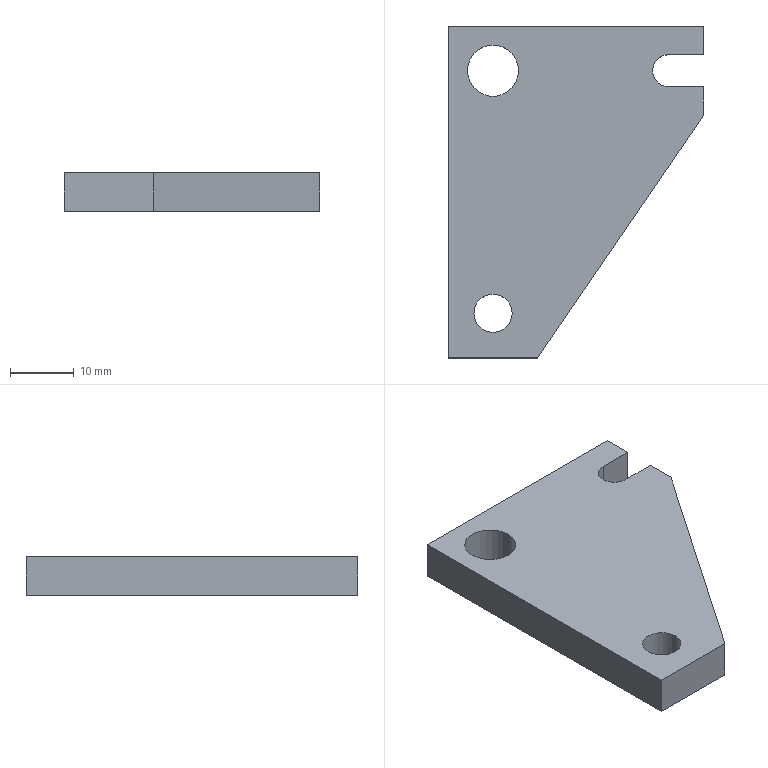Part | STEP file | BU-C03a | 1 solid | 16 faces | box 40 x 52 x 6 mm | volume 8821 mm3 | plane 10 | cylinder 6 | commonest cylinder face diameters 5 x2 6 x2 8 x2
STEP:
#1=CARTESIAN_POINT('',(0.,0.,0.));
#2=DIRECTION('',(0.,0.,1.));
#3=DIRECTION('',(1.,0.,0.));
#4=AXIS2_PLACEMENT_3D('',#1,#2,#3);
#5=CARTESIAN_POINT('',(3.,45.,6.));
#6=VERTEX_POINT('',#5);
#7=CARTESIAN_POINT('',(3.,45.,0.));
#8=VERTEX_POINT('',#7);
#9=CARTESIAN_POINT('',(3.,45.,6.));
#10=DIRECTION('',(0.,0.,-1.));
#11=VECTOR('',#10,1.);
#12=LINE('',#9,#11);
#13=CARTESIAN_POINT('',(7.,45.,6.));
#14=DIRECTION('',(0.,0.,-1.));
#15=DIRECTION('',(-1.,0.,0.));
#16=AXIS2_PLACEMENT_3D('',#13,#14,#15);
#17=CYLINDRICAL_SURFACE('',#16,4.);
#18=CARTESIAN_POINT('',(6.283,0.));
#19=DIRECTION('',(0.,1.));
#20=VECTOR('',#19,1.);
#21=LINE('',#18,#20);
#22=(GEOMETRIC_REPRESENTATION_CONTEXT(2)PARAMETRIC_REPRESENTATION_CONTEXT()REPRESENTATION_CONTEXT('',''));
#23=DEFINITIONAL_REPRESENTATION('',(#21),#22);
#24=PCURVE('',#17,#23);
#25=CARTESIAN_POINT('',(7.,45.,6.));
#26=DIRECTION('',(0.,0.,-1.));
#27=DIRECTION('',(-1.,0.,0.));
#28=AXIS2_PLACEMENT_3D('',#25,#26,#27);
#29=CYLINDRICAL_SURFACE('',#28,4.);
#30=CARTESIAN_POINT('',(0.,0.));
#31=DIRECTION('',(0.,1.));
#32=VECTOR('',#31,1.);
#33=LINE('',#30,#32);
#34=(GEOMETRIC_REPRESENTATION_CONTEXT(2)PARAMETRIC_REPRESENTATION_CONTEXT()REPRESENTATION_CONTEXT('',''));
#35=DEFINITIONAL_REPRESENTATION('',(#33),#34);
#36=PCURVE('',#29,#35);
#37=SURFACE_CURVE('',#12,(#24,#36),.PCURVE_S1.);
#38=EDGE_CURVE('',#6,#8,#37,.T.);
#39=ORIENTED_EDGE('',*,*,#38,.T.);
#40=CARTESIAN_POINT('',(11.,45.,0.));
#41=VERTEX_POINT('',#40);
#42=CARTESIAN_POINT('',(7.,45.,0.));
#43=DIRECTION('',(0.,0.,1.));
#44=DIRECTION('',(1.,0.,0.));
#45=AXIS2_PLACEMENT_3D('',#42,#43,#44);
#46=CIRCLE('',#45,4.);
#47=CARTESIAN_POINT('',(9.425,6.));
#48=DIRECTION('',(-1.,0.));
#49=VECTOR('',#48,1.);
#50=LINE('',#47,#49);
#51=(GEOMETRIC_REPRESENTATION_CONTEXT(2)PARAMETRIC_REPRESENTATION_CONTEXT()REPRESENTATION_CONTEXT('',''));
#52=DEFINITIONAL_REPRESENTATION('',(#50),#51);
#53=PCURVE('',#17,#52);
#54=CARTESIAN_POINT('',(34.5,45.,0.));
#55=DIRECTION('',(0.,0.,1.));
#56=DIRECTION('',(1.,0.,0.));
#57=AXIS2_PLACEMENT_3D('',#54,#55,#56);
#58=PLANE('',#57);
#59=CARTESIAN_POINT('',(-27.5,0.));
#60=DIRECTION('',(1.,0.));
#61=AXIS2_PLACEMENT_2D('',#59,#60);
#62=CIRCLE('',#61,4.);
#63=(GEOMETRIC_REPRESENTATION_CONTEXT(2)PARAMETRIC_REPRESENTATION_CONTEXT()REPRESENTATION_CONTEXT('',''));
#64=DEFINITIONAL_REPRESENTATION('',(#62),#63);
#65=PCURVE('',#58,#64);
#66=SURFACE_CURVE('',#46,(#53,#65),.PCURVE_S1.);
#67=EDGE_CURVE('',#8,#41,#66,.T.);
#68=ORIENTED_EDGE('',*,*,#67,.T.);
#69=CARTESIAN_POINT('',(11.,45.,6.));
#70=VERTEX_POINT('',#69);
#71=CARTESIAN_POINT('',(11.,45.,6.));
#72=DIRECTION('',(0.,0.,-1.));
#73=VECTOR('',#72,1.);
#74=LINE('',#71,#73);
#75=CARTESIAN_POINT('',(3.142,0.));
#76=DIRECTION('',(0.,1.));
#77=VECTOR('',#76,1.);
#78=LINE('',#75,#77);
#79=(GEOMETRIC_REPRESENTATION_CONTEXT(2)PARAMETRIC_REPRESENTATION_CONTEXT()REPRESENTATION_CONTEXT('',''));
#80=DEFINITIONAL_REPRESENTATION('',(#78),#79);
#81=PCURVE('',#17,#80);
#82=CARTESIAN_POINT('',(3.142,0.));
#83=DIRECTION('',(0.,1.));
#84=VECTOR('',#83,1.);
#85=LINE('',#82,#84);
#86=(GEOMETRIC_REPRESENTATION_CONTEXT(2)PARAMETRIC_REPRESENTATION_CONTEXT()REPRESENTATION_CONTEXT('',''));
#87=DEFINITIONAL_REPRESENTATION('',(#85),#86);
#88=PCURVE('',#29,#87);
#89=SURFACE_CURVE('',#74,(#81,#88),.PCURVE_S1.);
#90=EDGE_CURVE('',#70,#41,#89,.T.);
#91=ORIENTED_EDGE('',*,*,#90,.F.);
#92=CARTESIAN_POINT('',(7.,45.,6.));
#93=DIRECTION('',(0.,0.,1.));
#94=DIRECTION('',(1.,0.,0.));
#95=AXIS2_PLACEMENT_3D('',#92,#93,#94);
#96=CIRCLE('',#95,4.);
#97=CARTESIAN_POINT('',(9.425,0.));
#98=DIRECTION('',(-1.,0.));
#99=VECTOR('',#98,1.);
#100=LINE('',#97,#99);
#101=(GEOMETRIC_REPRESENTATION_CONTEXT(2)PARAMETRIC_REPRESENTATION_CONTEXT()REPRESENTATION_CONTEXT('',''));
#102=DEFINITIONAL_REPRESENTATION('',(#100),#101);
#103=PCURVE('',#17,#102);
#104=CARTESIAN_POINT('',(34.5,45.,6.));
#105=DIRECTION('',(0.,0.,1.));
#106=DIRECTION('',(1.,0.,0.));
#107=AXIS2_PLACEMENT_3D('',#104,#105,#106);
#108=PLANE('',#107);
#109=CARTESIAN_POINT('',(-27.5,0.));
#110=DIRECTION('',(1.,0.));
#111=AXIS2_PLACEMENT_2D('',#109,#110);
#112=CIRCLE('',#111,4.);
#113=(GEOMETRIC_REPRESENTATION_CONTEXT(2)PARAMETRIC_REPRESENTATION_CONTEXT()REPRESENTATION_CONTEXT('',''));
#114=DEFINITIONAL_REPRESENTATION('',(#112),#113);
#115=PCURVE('',#108,#114);
#116=SURFACE_CURVE('',#96,(#103,#115),.PCURVE_S1.);
#117=EDGE_CURVE('',#6,#70,#116,.T.);
#118=ORIENTED_EDGE('',*,*,#117,.F.);
#119=EDGE_LOOP('',(#39,#68,#91,#118));
#120=FACE_BOUND('',#119,.F.);
#121=ADVANCED_FACE('',(#120),#17,.F.);
#122=CARTESIAN_POINT('',(4.,7.,6.));
#123=VERTEX_POINT('',#122);
#124=CARTESIAN_POINT('',(4.,7.,0.));
#125=VERTEX_POINT('',#124);
#126=CARTESIAN_POINT('',(4.,7.,6.));
#127=DIRECTION('',(0.,0.,-1.));
#128=VECTOR('',#127,1.);
#129=LINE('',#126,#128);
#130=CARTESIAN_POINT('',(7.,7.,6.));
#131=DIRECTION('',(0.,0.,-1.));
#132=DIRECTION('',(-1.,0.,0.));
#133=AXIS2_PLACEMENT_3D('',#130,#131,#132);
#134=CYLINDRICAL_SURFACE('',#133,3.);
#135=CARTESIAN_POINT('',(6.283,0.));
#136=DIRECTION('',(0.,1.));
#137=VECTOR('',#136,1.);
#138=LINE('',#135,#137);
#139=(GEOMETRIC_REPRESENTATION_CONTEXT(2)PARAMETRIC_REPRESENTATION_CONTEXT()REPRESENTATION_CONTEXT('',''));
#140=DEFINITIONAL_REPRESENTATION('',(#138),#139);
#141=PCURVE('',#134,#140);
#142=CARTESIAN_POINT('',(7.,7.,6.));
#143=DIRECTION('',(0.,0.,-1.));
#144=DIRECTION('',(-1.,0.,0.));
#145=AXIS2_PLACEMENT_3D('',#142,#143,#144);
#146=CYLINDRICAL_SURFACE('',#145,3.);
#147=CARTESIAN_POINT('',(0.,0.));
#148=DIRECTION('',(0.,1.));
#149=VECTOR('',#148,1.);
#150=LINE('',#147,#149);
#151=(GEOMETRIC_REPRESENTATION_CONTEXT(2)PARAMETRIC_REPRESENTATION_CONTEXT()REPRESENTATION_CONTEXT('',''));
#152=DEFINITIONAL_REPRESENTATION('',(#150),#151);
#153=PCURVE('',#146,#152);
#154=SURFACE_CURVE('',#129,(#141,#153),.PCURVE_S1.);
#155=EDGE_CURVE('',#123,#125,#154,.T.);
#156=ORIENTED_EDGE('',*,*,#155,.T.);
#157=CARTESIAN_POINT('',(10.,7.,0.));
#158=VERTEX_POINT('',#157);
#159=CARTESIAN_POINT('',(7.,7.,0.));
#160=DIRECTION('',(0.,0.,1.));
#161=DIRECTION('',(1.,0.,0.));
#162=AXIS2_PLACEMENT_3D('',#159,#160,#161);
#163=CIRCLE('',#162,3.);
#164=CARTESIAN_POINT('',(9.425,6.));
#165=DIRECTION('',(-1.,0.));
#166=VECTOR('',#165,1.);
#167=LINE('',#164,#166);
#168=(GEOMETRIC_REPRESENTATION_CONTEXT(2)PARAMETRIC_REPRESENTATION_CONTEXT()REPRESENTATION_CONTEXT('',''));
#169=DEFINITIONAL_REPRESENTATION('',(#167),#168);
#170=PCURVE('',#134,#169);
#171=CARTESIAN_POINT('',(-27.5,-38.));
#172=DIRECTION('',(1.,0.));
#173=AXIS2_PLACEMENT_2D('',#171,#172);
#174=CIRCLE('',#173,3.);
#175=(GEOMETRIC_REPRESENTATION_CONTEXT(2)PARAMETRIC_REPRESENTATION_CONTEXT()REPRESENTATION_CONTEXT('',''));
#176=DEFINITIONAL_REPRESENTATION('',(#174),#175);
#177=PCURVE('',#58,#176);
#178=SURFACE_CURVE('',#163,(#170,#177),.PCURVE_S1.);
#179=EDGE_CURVE('',#125,#158,#178,.T.);
#180=ORIENTED_EDGE('',*,*,#179,.T.);
#181=CARTESIAN_POINT('',(10.,7.,6.));
#182=VERTEX_POINT('',#181);
#183=CARTESIAN_POINT('',(10.,7.,6.));
#184=DIRECTION('',(0.,0.,-1.));
#185=VECTOR('',#184,1.);
#186=LINE('',#183,#185);
#187=CARTESIAN_POINT('',(3.142,0.));
#188=DIRECTION('',(0.,1.));
#189=VECTOR('',#188,1.);
#190=LINE('',#187,#189);
#191=(GEOMETRIC_REPRESENTATION_CONTEXT(2)PARAMETRIC_REPRESENTATION_CONTEXT()REPRESENTATION_CONTEXT('',''));
#192=DEFINITIONAL_REPRESENTATION('',(#190),#191);
#193=PCURVE('',#134,#192);
#194=CARTESIAN_POINT('',(3.142,0.));
#195=DIRECTION('',(0.,1.));
#196=VECTOR('',#195,1.);
#197=LINE('',#194,#196);
#198=(GEOMETRIC_REPRESENTATION_CONTEXT(2)PARAMETRIC_REPRESENTATION_CONTEXT()REPRESENTATION_CONTEXT('',''));
#199=DEFINITIONAL_REPRESENTATION('',(#197),#198);
#200=PCURVE('',#146,#199);
#201=SURFACE_CURVE('',#186,(#193,#200),.PCURVE_S1.);
#202=EDGE_CURVE('',#182,#158,#201,.T.);
#203=ORIENTED_EDGE('',*,*,#202,.F.);
#204=CARTESIAN_POINT('',(7.,7.,6.));
#205=DIRECTION('',(0.,0.,1.));
#206=DIRECTION('',(1.,0.,0.));
#207=AXIS2_PLACEMENT_3D('',#204,#205,#206);
#208=CIRCLE('',#207,3.);
#209=CARTESIAN_POINT('',(9.425,0.));
#210=DIRECTION('',(-1.,0.));
#211=VECTOR('',#210,1.);
#212=LINE('',#209,#211);
#213=(GEOMETRIC_REPRESENTATION_CONTEXT(2)PARAMETRIC_REPRESENTATION_CONTEXT()REPRESENTATION_CONTEXT('',''));
#214=DEFINITIONAL_REPRESENTATION('',(#212),#213);
#215=PCURVE('',#134,#214);
#216=CARTESIAN_POINT('',(-27.5,-38.));
#217=DIRECTION('',(1.,0.));
#218=AXIS2_PLACEMENT_2D('',#216,#217);
#219=CIRCLE('',#218,3.);
#220=(GEOMETRIC_REPRESENTATION_CONTEXT(2)PARAMETRIC_REPRESENTATION_CONTEXT()REPRESENTATION_CONTEXT('',''));
#221=DEFINITIONAL_REPRESENTATION('',(#219),#220);
#222=PCURVE('',#108,#221);
#223=SURFACE_CURVE('',#208,(#215,#222),.PCURVE_S1.);
#224=EDGE_CURVE('',#123,#182,#223,.T.);
#225=ORIENTED_EDGE('',*,*,#224,.F.);
#226=EDGE_LOOP('',(#156,#180,#203,#225));
#227=FACE_BOUND('',#226,.F.);
#228=ADVANCED_FACE('',(#227),#134,.F.);
#229=CARTESIAN_POINT('',(34.5,47.5,6.));
#230=VERTEX_POINT('',#229);
#231=CARTESIAN_POINT('',(34.5,47.5,0.));
#232=VERTEX_POINT('',#231);
#233=CARTESIAN_POINT('',(34.5,47.5,6.));
#234=DIRECTION('',(0.,0.,-1.));
#235=VECTOR('',#234,1.);
#236=LINE('',#233,#235);
#237=CARTESIAN_POINT('',(34.5,45.,6.));
#238=DIRECTION('',(0.,0.,-1.));
#239=DIRECTION('',(-1.,0.,0.));
#240=AXIS2_PLACEMENT_3D('',#237,#238,#239);
#241=CYLINDRICAL_SURFACE('',#240,2.5);
#242=CARTESIAN_POINT('',(1.571,0.));
#243=DIRECTION('',(0.,1.));
#244=VECTOR('',#243,1.);
#245=LINE('',#242,#244);
#246=(GEOMETRIC_REPRESENTATION_CONTEXT(2)PARAMETRIC_REPRESENTATION_CONTEXT()REPRESENTATION_CONTEXT('',''));
#247=DEFINITIONAL_REPRESENTATION('',(#245),#246);
#248=PCURVE('',#241,#247);
#249=CARTESIAN_POINT('',(40.,47.5,6.));
#250=DIRECTION('',(0.,1.,0.));
#251=DIRECTION('',(0.,0.,1.));
#252=AXIS2_PLACEMENT_3D('',#249,#250,#251);
#253=PLANE('',#252);
#254=CARTESIAN_POINT('',(0.,-5.5));
#255=DIRECTION('',(-1.,0.));
#256=VECTOR('',#255,1.);
#257=LINE('',#254,#256);
#258=(GEOMETRIC_REPRESENTATION_CONTEXT(2)PARAMETRIC_REPRESENTATION_CONTEXT()REPRESENTATION_CONTEXT('',''));
#259=DEFINITIONAL_REPRESENTATION('',(#257),#258);
#260=PCURVE('',#253,#259);
#261=SURFACE_CURVE('',#236,(#248,#260),.PCURVE_S1.);
#262=EDGE_CURVE('',#230,#232,#261,.T.);
#263=ORIENTED_EDGE('',*,*,#262,.T.);
#264=CARTESIAN_POINT('',(32.,45.,0.));
#265=VERTEX_POINT('',#264);
#266=CARTESIAN_POINT('',(34.5,45.,0.));
#267=DIRECTION('',(0.,0.,-1.));
#268=DIRECTION('',(1.,0.,0.));
#269=AXIS2_PLACEMENT_3D('',#266,#267,#268);
#270=CIRCLE('',#269,2.5);
#271=CARTESIAN_POINT('',(-3.142,6.));
#272=DIRECTION('',(1.,0.));
#273=VECTOR('',#272,1.);
#274=LINE('',#271,#273);
#275=(GEOMETRIC_REPRESENTATION_CONTEXT(2)PARAMETRIC_REPRESENTATION_CONTEXT()REPRESENTATION_CONTEXT('',''));
#276=DEFINITIONAL_REPRESENTATION('',(#274),#275);
#277=PCURVE('',#241,#276);
#278=CARTESIAN_POINT('',(2.5,0.));
#279=CARTESIAN_POINT('',(2.5,-4.33));
#280=CARTESIAN_POINT('',(-1.25,-2.165));
#281=CARTESIAN_POINT('',(-5.,0.));
#282=CARTESIAN_POINT('',(-1.25,2.165));
#283=CARTESIAN_POINT('',(2.5,4.33));
#284=CARTESIAN_POINT('',(2.5,0.));
#285=(BOUNDED_CURVE()B_SPLINE_CURVE(2,(#278,#279,#280,#281,#282,#283,#284),.UNSPECIFIED.,.T.,.F.)B_SPLINE_CURVE_WITH_KNOTS((1,2,2,2,2,1),(-2.094,0.,2.094,4.189,6.283,8.378),.UNSPECIFIED.)CURVE()GEOMETRIC_REPRESENTATION_ITEM()RATIONAL_B_SPLINE_CURVE((1.,0.5,1.,0.5,1.,0.5,1.))REPRESENTATION_ITEM(''));
#286=(GEOMETRIC_REPRESENTATION_CONTEXT(2)PARAMETRIC_REPRESENTATION_CONTEXT()REPRESENTATION_CONTEXT('',''));
#287=DEFINITIONAL_REPRESENTATION('',(#285),#286);
#288=PCURVE('',#58,#287);
#289=SURFACE_CURVE('',#270,(#277,#288),.PCURVE_S1.);
#290=EDGE_CURVE('',#265,#232,#289,.T.);
#291=ORIENTED_EDGE('',*,*,#290,.F.);
#292=CARTESIAN_POINT('',(32.,45.,6.));
#293=VERTEX_POINT('',#292);
#294=CARTESIAN_POINT('',(32.,45.,6.));
#295=DIRECTION('',(0.,0.,-1.));
#296=VECTOR('',#295,1.);
#297=LINE('',#294,#296);
#298=CARTESIAN_POINT('',(0.,0.));
#299=DIRECTION('',(0.,1.));
#300=VECTOR('',#299,1.);
#301=LINE('',#298,#300);
#302=(GEOMETRIC_REPRESENTATION_CONTEXT(2)PARAMETRIC_REPRESENTATION_CONTEXT()REPRESENTATION_CONTEXT('',''));
#303=DEFINITIONAL_REPRESENTATION('',(#301),#302);
#304=PCURVE('',#241,#303);
#305=CARTESIAN_POINT('',(34.5,45.,6.));
#306=DIRECTION('',(0.,0.,-1.));
#307=DIRECTION('',(-1.,0.,0.));
#308=AXIS2_PLACEMENT_3D('',#305,#306,#307);
#309=CYLINDRICAL_SURFACE('',#308,2.5);
#310=CARTESIAN_POINT('',(6.283,0.));
#311=DIRECTION('',(0.,1.));
#312=VECTOR('',#311,1.);
#313=LINE('',#310,#312);
#314=(GEOMETRIC_REPRESENTATION_CONTEXT(2)PARAMETRIC_REPRESENTATION_CONTEXT()REPRESENTATION_CONTEXT('',''));
#315=DEFINITIONAL_REPRESENTATION('',(#313),#314);
#316=PCURVE('',#309,#315);
#317=SURFACE_CURVE('',#297,(#304,#316),.PCURVE_S1.);
#318=EDGE_CURVE('',#293,#265,#317,.T.);
#319=ORIENTED_EDGE('',*,*,#318,.F.);
#320=CARTESIAN_POINT('',(34.5,45.,6.));
#321=DIRECTION('',(0.,0.,-1.));
#322=DIRECTION('',(1.,0.,0.));
#323=AXIS2_PLACEMENT_3D('',#320,#321,#322);
#324=CIRCLE('',#323,2.5);
#325=CARTESIAN_POINT('',(-3.142,0.));
#326=DIRECTION('',(1.,0.));
#327=VECTOR('',#326,1.);
#328=LINE('',#325,#327);
#329=(GEOMETRIC_REPRESENTATION_CONTEXT(2)PARAMETRIC_REPRESENTATION_CONTEXT()REPRESENTATION_CONTEXT('',''));
#330=DEFINITIONAL_REPRESENTATION('',(#328),#329);
#331=PCURVE('',#241,#330);
#332=CARTESIAN_POINT('',(2.5,0.));
#333=CARTESIAN_POINT('',(2.5,-4.33));
#334=CARTESIAN_POINT('',(-1.25,-2.165));
#335=CARTESIAN_POINT('',(-5.,0.));
#336=CARTESIAN_POINT('',(-1.25,2.165));
#337=CARTESIAN_POINT('',(2.5,4.33));
#338=CARTESIAN_POINT('',(2.5,0.));
#339=(BOUNDED_CURVE()B_SPLINE_CURVE(2,(#332,#333,#334,#335,#336,#337,#338),.UNSPECIFIED.,.T.,.F.)B_SPLINE_CURVE_WITH_KNOTS((1,2,2,2,2,1),(-2.094,0.,2.094,4.189,6.283,8.378),.UNSPECIFIED.)CURVE()GEOMETRIC_REPRESENTATION_ITEM()RATIONAL_B_SPLINE_CURVE((1.,0.5,1.,0.5,1.,0.5,1.))REPRESENTATION_ITEM(''));
#340=(GEOMETRIC_REPRESENTATION_CONTEXT(2)PARAMETRIC_REPRESENTATION_CONTEXT()REPRESENTATION_CONTEXT('',''));
#341=DEFINITIONAL_REPRESENTATION('',(#339),#340);
#342=PCURVE('',#108,#341);
#343=SURFACE_CURVE('',#324,(#331,#342),.PCURVE_S1.);
#344=EDGE_CURVE('',#293,#230,#343,.T.);
#345=ORIENTED_EDGE('',*,*,#344,.T.);
#346=EDGE_LOOP('',(#263,#291,#319,#345));
#347=FACE_BOUND('',#346,.F.);
#348=ADVANCED_FACE('',(#347),#241,.F.);
#349=ORIENTED_EDGE('',*,*,#224,.F.);
#350=CARTESIAN_POINT('',(7.,7.,6.));
#351=DIRECTION('',(0.,0.,1.));
#352=DIRECTION('',(1.,0.,0.));
#353=AXIS2_PLACEMENT_3D('',#350,#351,#352);
#354=CIRCLE('',#353,3.);
#355=CARTESIAN_POINT('',(-27.5,-38.));
#356=DIRECTION('',(1.,0.));
#357=AXIS2_PLACEMENT_2D('',#355,#356);
#358=CIRCLE('',#357,3.);
#359=(GEOMETRIC_REPRESENTATION_CONTEXT(2)PARAMETRIC_REPRESENTATION_CONTEXT()REPRESENTATION_CONTEXT('',''));
#360=DEFINITIONAL_REPRESENTATION('',(#358),#359);
#361=PCURVE('',#108,#360);
#362=CARTESIAN_POINT('',(3.142,0.));
#363=DIRECTION('',(-1.,0.));
#364=VECTOR('',#363,1.);
#365=LINE('',#362,#364);
#366=(GEOMETRIC_REPRESENTATION_CONTEXT(2)PARAMETRIC_REPRESENTATION_CONTEXT()REPRESENTATION_CONTEXT('',''));
#367=DEFINITIONAL_REPRESENTATION('',(#365),#366);
#368=PCURVE('',#146,#367);
#369=SURFACE_CURVE('',#354,(#361,#368),.PCURVE_S1.);
#370=EDGE_CURVE('',#182,#123,#369,.T.);
#371=ORIENTED_EDGE('',*,*,#370,.F.);
#372=EDGE_LOOP('',(#349,#371));
#373=FACE_BOUND('',#372,.T.);
#374=CARTESIAN_POINT('',(40.,47.5,6.));
#375=VERTEX_POINT('',#374);
#376=CARTESIAN_POINT('',(40.,47.5,6.));
#377=DIRECTION('',(1.,0.,0.));
#378=VECTOR('',#377,1.);
#379=LINE('',#376,#378);
#380=CARTESIAN_POINT('',(5.5,2.5));
#381=DIRECTION('',(1.,0.));
#382=VECTOR('',#381,1.);
#383=LINE('',#380,#382);
#384=(GEOMETRIC_REPRESENTATION_CONTEXT(2)PARAMETRIC_REPRESENTATION_CONTEXT()REPRESENTATION_CONTEXT('',''));
#385=DEFINITIONAL_REPRESENTATION('',(#383),#384);
#386=PCURVE('',#108,#385);
#387=CARTESIAN_POINT('',(0.,0.));
#388=DIRECTION('',(0.,1.));
#389=VECTOR('',#388,1.);
#390=LINE('',#387,#389);
#391=(GEOMETRIC_REPRESENTATION_CONTEXT(2)PARAMETRIC_REPRESENTATION_CONTEXT()REPRESENTATION_CONTEXT('',''));
#392=DEFINITIONAL_REPRESENTATION('',(#390),#391);
#393=PCURVE('',#253,#392);
#394=SURFACE_CURVE('',#379,(#386,#393),.PCURVE_S1.);
#395=EDGE_CURVE('',#230,#375,#394,.T.);
#396=ORIENTED_EDGE('',*,*,#395,.T.);
#397=CARTESIAN_POINT('',(40.,52.,6.));
#398=VERTEX_POINT('',#397);
#399=CARTESIAN_POINT('',(40.,47.5,6.));
#400=DIRECTION('',(0.,1.,0.));
#401=VECTOR('',#400,1.);
#402=LINE('',#399,#401);
#403=CARTESIAN_POINT('',(5.5,2.5));
#404=DIRECTION('',(0.,1.));
#405=VECTOR('',#404,1.);
#406=LINE('',#403,#405);
#407=(GEOMETRIC_REPRESENTATION_CONTEXT(2)PARAMETRIC_REPRESENTATION_CONTEXT()REPRESENTATION_CONTEXT('',''));
#408=DEFINITIONAL_REPRESENTATION('',(#406),#407);
#409=PCURVE('',#108,#408);
#410=CARTESIAN_POINT('',(40.,47.5,6.));
#411=DIRECTION('',(-1.,0.,0.));
#412=DIRECTION('',(0.,0.,1.));
#413=AXIS2_PLACEMENT_3D('',#410,#411,#412);
#414=PLANE('',#413);
#415=CARTESIAN_POINT('',(0.,0.));
#416=DIRECTION('',(0.,1.));
#417=VECTOR('',#416,1.);
#418=LINE('',#415,#417);
#419=(GEOMETRIC_REPRESENTATION_CONTEXT(2)PARAMETRIC_REPRESENTATION_CONTEXT()REPRESENTATION_CONTEXT('',''));
#420=DEFINITIONAL_REPRESENTATION('',(#418),#419);
#421=PCURVE('',#414,#420);
#422=SURFACE_CURVE('',#402,(#409,#421),.PCURVE_S1.);
#423=EDGE_CURVE('',#375,#398,#422,.T.);
#424=ORIENTED_EDGE('',*,*,#423,.T.);
#425=CARTESIAN_POINT('',(0.,52.,6.));
#426=VERTEX_POINT('',#425);
#427=CARTESIAN_POINT('',(40.,52.,6.));
#428=DIRECTION('',(-1.,0.,0.));
#429=VECTOR('',#428,1.);
#430=LINE('',#427,#429);
#431=CARTESIAN_POINT('',(5.5,7.));
#432=DIRECTION('',(-1.,0.));
#433=VECTOR('',#432,1.);
#434=LINE('',#431,#433);
#435=(GEOMETRIC_REPRESENTATION_CONTEXT(2)PARAMETRIC_REPRESENTATION_CONTEXT()REPRESENTATION_CONTEXT('',''));
#436=DEFINITIONAL_REPRESENTATION('',(#434),#435);
#437=PCURVE('',#108,#436);
#438=CARTESIAN_POINT('',(40.,52.,6.));
#439=DIRECTION('',(0.,-1.,0.));
#440=DIRECTION('',(0.,0.,-1.));
#441=AXIS2_PLACEMENT_3D('',#438,#439,#440);
#442=PLANE('',#441);
#443=CARTESIAN_POINT('',(0.,0.));
#444=DIRECTION('',(0.,-1.));
#445=VECTOR('',#444,1.);
#446=LINE('',#443,#445);
#447=(GEOMETRIC_REPRESENTATION_CONTEXT(2)PARAMETRIC_REPRESENTATION_CONTEXT()REPRESENTATION_CONTEXT('',''));
#448=DEFINITIONAL_REPRESENTATION('',(#446),#447);
#449=PCURVE('',#442,#448);
#450=SURFACE_CURVE('',#430,(#437,#449),.PCURVE_S1.);
#451=EDGE_CURVE('',#398,#426,#450,.T.);
#452=ORIENTED_EDGE('',*,*,#451,.T.);
#453=CARTESIAN_POINT('',(0.,0.,6.));
#454=VERTEX_POINT('',#453);
#455=CARTESIAN_POINT('',(0.,0.,6.));
#456=DIRECTION('',(0.,-1.,0.));
#457=VECTOR('',#456,1.);
#458=LINE('',#455,#457);
#459=CARTESIAN_POINT('',(-34.5,-45.));
#460=DIRECTION('',(0.,-1.));
#461=VECTOR('',#460,1.);
#462=LINE('',#459,#461);
#463=(GEOMETRIC_REPRESENTATION_CONTEXT(2)PARAMETRIC_REPRESENTATION_CONTEXT()REPRESENTATION_CONTEXT('',''));
#464=DEFINITIONAL_REPRESENTATION('',(#462),#463);
#465=PCURVE('',#108,#464);
#466=CARTESIAN_POINT('',(0.,0.,6.));
#467=DIRECTION('',(1.,0.,0.));
#468=DIRECTION('',(0.,0.,-1.));
#469=AXIS2_PLACEMENT_3D('',#466,#467,#468);
#470=PLANE('',#469);
#471=CARTESIAN_POINT('',(0.,0.));
#472=DIRECTION('',(0.,-1.));
#473=VECTOR('',#472,1.);
#474=LINE('',#471,#473);
#475=(GEOMETRIC_REPRESENTATION_CONTEXT(2)PARAMETRIC_REPRESENTATION_CONTEXT()REPRESENTATION_CONTEXT('',''));
#476=DEFINITIONAL_REPRESENTATION('',(#474),#475);
#477=PCURVE('',#470,#476);
#478=SURFACE_CURVE('',#458,(#465,#477),.PCURVE_S1.);
#479=EDGE_CURVE('',#426,#454,#478,.T.);
#480=ORIENTED_EDGE('',*,*,#479,.T.);
#481=CARTESIAN_POINT('',(14.,0.,6.));
#482=VERTEX_POINT('',#481);
#483=CARTESIAN_POINT('',(14.,0.,6.));
#484=DIRECTION('',(1.,0.,0.));
#485=VECTOR('',#484,1.);
#486=LINE('',#483,#485);
#487=CARTESIAN_POINT('',(-20.5,-45.));
#488=DIRECTION('',(1.,0.));
#489=VECTOR('',#488,1.);
#490=LINE('',#487,#489);
#491=(GEOMETRIC_REPRESENTATION_CONTEXT(2)PARAMETRIC_REPRESENTATION_CONTEXT()REPRESENTATION_CONTEXT('',''));
#492=DEFINITIONAL_REPRESENTATION('',(#490),#491);
#493=PCURVE('',#108,#492);
#494=CARTESIAN_POINT('',(14.,0.,6.));
#495=DIRECTION('',(0.,1.,0.));
#496=DIRECTION('',(0.,0.,1.));
#497=AXIS2_PLACEMENT_3D('',#494,#495,#496);
#498=PLANE('',#497);
#499=CARTESIAN_POINT('',(0.,0.));
#500=DIRECTION('',(0.,1.));
#501=VECTOR('',#500,1.);
#502=LINE('',#499,#501);
#503=(GEOMETRIC_REPRESENTATION_CONTEXT(2)PARAMETRIC_REPRESENTATION_CONTEXT()REPRESENTATION_CONTEXT('',''));
#504=DEFINITIONAL_REPRESENTATION('',(#502),#503);
#505=PCURVE('',#498,#504);
#506=SURFACE_CURVE('',#486,(#493,#505),.PCURVE_S1.);
#507=EDGE_CURVE('',#454,#482,#506,.T.);
#508=ORIENTED_EDGE('',*,*,#507,.T.);
#509=CARTESIAN_POINT('',(40.,38.,6.));
#510=VERTEX_POINT('',#509);
#511=CARTESIAN_POINT('',(14.,0.,6.));
#512=DIRECTION('',(0.5647,0.8253,0.));
#513=VECTOR('',#512,1.);
#514=LINE('',#511,#513);
#515=CARTESIAN_POINT('',(-20.5,-45.));
#516=DIRECTION('',(0.5647,0.8253));
#517=VECTOR('',#516,1.);
#518=LINE('',#515,#517);
#519=(GEOMETRIC_REPRESENTATION_CONTEXT(2)PARAMETRIC_REPRESENTATION_CONTEXT()REPRESENTATION_CONTEXT('',''));
#520=DEFINITIONAL_REPRESENTATION('',(#518),#519);
#521=PCURVE('',#108,#520);
#522=CARTESIAN_POINT('',(14.,0.,6.));
#523=DIRECTION('',(-0.8253,0.5647,0.));
#524=DIRECTION('',(-0.5647,-0.8253,0.));
#525=AXIS2_PLACEMENT_3D('',#522,#523,#524);
#526=PLANE('',#525);
#527=CARTESIAN_POINT('',(0.,0.));
#528=DIRECTION('',(-1.,0.));
#529=VECTOR('',#528,1.);
#530=LINE('',#527,#529);
#531=(GEOMETRIC_REPRESENTATION_CONTEXT(2)PARAMETRIC_REPRESENTATION_CONTEXT()REPRESENTATION_CONTEXT('',''));
#532=DEFINITIONAL_REPRESENTATION('',(#530),#531);
#533=PCURVE('',#526,#532);
#534=SURFACE_CURVE('',#514,(#521,#533),.PCURVE_S1.);
#535=EDGE_CURVE('',#482,#510,#534,.T.);
#536=ORIENTED_EDGE('',*,*,#535,.T.);
#537=CARTESIAN_POINT('',(40.,42.5,6.));
#538=VERTEX_POINT('',#537);
#539=CARTESIAN_POINT('',(40.,38.,6.));
#540=DIRECTION('',(0.,1.,0.));
#541=VECTOR('',#540,1.);
#542=LINE('',#539,#541);
#543=CARTESIAN_POINT('',(5.5,-7.));
#544=DIRECTION('',(0.,1.));
#545=VECTOR('',#544,1.);
#546=LINE('',#543,#545);
#547=(GEOMETRIC_REPRESENTATION_CONTEXT(2)PARAMETRIC_REPRESENTATION_CONTEXT()REPRESENTATION_CONTEXT('',''));
#548=DEFINITIONAL_REPRESENTATION('',(#546),#547);
#549=PCURVE('',#108,#548);
#550=CARTESIAN_POINT('',(40.,38.,6.));
#551=DIRECTION('',(-1.,0.,0.));
#552=DIRECTION('',(0.,0.,1.));
#553=AXIS2_PLACEMENT_3D('',#550,#551,#552);
#554=PLANE('',#553);
#555=CARTESIAN_POINT('',(0.,0.));
#556=DIRECTION('',(0.,1.));
#557=VECTOR('',#556,1.);
#558=LINE('',#555,#557);
#559=(GEOMETRIC_REPRESENTATION_CONTEXT(2)PARAMETRIC_REPRESENTATION_CONTEXT()REPRESENTATION_CONTEXT('',''));
#560=DEFINITIONAL_REPRESENTATION('',(#558),#559);
#561=PCURVE('',#554,#560);
#562=SURFACE_CURVE('',#542,(#549,#561),.PCURVE_S1.);
#563=EDGE_CURVE('',#510,#538,#562,.T.);
#564=ORIENTED_EDGE('',*,*,#563,.T.);
#565=CARTESIAN_POINT('',(34.5,42.5,6.));
#566=VERTEX_POINT('',#565);
#567=CARTESIAN_POINT('',(40.,42.5,6.));
#568=DIRECTION('',(-1.,0.,0.));
#569=VECTOR('',#568,1.);
#570=LINE('',#567,#569);
#571=CARTESIAN_POINT('',(5.5,-2.5));
#572=DIRECTION('',(-1.,0.));
#573=VECTOR('',#572,1.);
#574=LINE('',#571,#573);
#575=(GEOMETRIC_REPRESENTATION_CONTEXT(2)PARAMETRIC_REPRESENTATION_CONTEXT()REPRESENTATION_CONTEXT('',''));
#576=DEFINITIONAL_REPRESENTATION('',(#574),#575);
#577=PCURVE('',#108,#576);
#578=CARTESIAN_POINT('',(40.,42.5,6.));
#579=DIRECTION('',(0.,-1.,0.));
#580=DIRECTION('',(0.,0.,-1.));
#581=AXIS2_PLACEMENT_3D('',#578,#579,#580);
#582=PLANE('',#581);
#583=CARTESIAN_POINT('',(0.,0.));
#584=DIRECTION('',(0.,-1.));
#585=VECTOR('',#584,1.);
#586=LINE('',#583,#585);
#587=(GEOMETRIC_REPRESENTATION_CONTEXT(2)PARAMETRIC_REPRESENTATION_CONTEXT()REPRESENTATION_CONTEXT('',''));
#588=DEFINITIONAL_REPRESENTATION('',(#586),#587);
#589=PCURVE('',#582,#588);
#590=SURFACE_CURVE('',#570,(#577,#589),.PCURVE_S1.);
#591=EDGE_CURVE('',#538,#566,#590,.T.);
#592=ORIENTED_EDGE('',*,*,#591,.T.);
#593=CARTESIAN_POINT('',(34.5,45.,6.));
#594=DIRECTION('',(0.,0.,-1.));
#595=DIRECTION('',(1.,0.,0.));
#596=AXIS2_PLACEMENT_3D('',#593,#594,#595);
#597=CIRCLE('',#596,2.5);
#598=CARTESIAN_POINT('',(2.5,0.));
#599=CARTESIAN_POINT('',(2.5,-4.33));
#600=CARTESIAN_POINT('',(-1.25,-2.165));
#601=CARTESIAN_POINT('',(-5.,0.));
#602=CARTESIAN_POINT('',(-1.25,2.165));
#603=CARTESIAN_POINT('',(2.5,4.33));
#604=CARTESIAN_POINT('',(2.5,0.));
#605=(BOUNDED_CURVE()B_SPLINE_CURVE(2,(#598,#599,#600,#601,#602,#603,#604),.UNSPECIFIED.,.T.,.F.)B_SPLINE_CURVE_WITH_KNOTS((1,2,2,2,2,1),(-2.094,0.,2.094,4.189,6.283,8.378),.UNSPECIFIED.)CURVE()GEOMETRIC_REPRESENTATION_ITEM()RATIONAL_B_SPLINE_CURVE((1.,0.5,1.,0.5,1.,0.5,1.))REPRESENTATION_ITEM(''));
#606=(GEOMETRIC_REPRESENTATION_CONTEXT(2)PARAMETRIC_REPRESENTATION_CONTEXT()REPRESENTATION_CONTEXT('',''));
#607=DEFINITIONAL_REPRESENTATION('',(#605),#606);
#608=PCURVE('',#108,#607);
#609=CARTESIAN_POINT('',(3.142,0.));
#610=DIRECTION('',(1.,0.));
#611=VECTOR('',#610,1.);
#612=LINE('',#609,#611);
#613=(GEOMETRIC_REPRESENTATION_CONTEXT(2)PARAMETRIC_REPRESENTATION_CONTEXT()REPRESENTATION_CONTEXT('',''));
#614=DEFINITIONAL_REPRESENTATION('',(#612),#613);
#615=PCURVE('',#309,#614);
#616=SURFACE_CURVE('',#597,(#608,#615),.PCURVE_S1.);
#617=EDGE_CURVE('',#566,#293,#616,.T.);
#618=ORIENTED_EDGE('',*,*,#617,.T.);
#619=ORIENTED_EDGE('',*,*,#344,.T.);
#620=EDGE_LOOP('',(#396,#424,#452,#480,#508,#536,#564,#592,#618,#619));
#621=FACE_BOUND('',#620,.T.);
#622=ORIENTED_EDGE('',*,*,#117,.F.);
#623=CARTESIAN_POINT('',(7.,45.,6.));
#624=DIRECTION('',(0.,0.,1.));
#625=DIRECTION('',(1.,0.,0.));
#626=AXIS2_PLACEMENT_3D('',#623,#624,#625);
#627=CIRCLE('',#626,4.);
#628=CARTESIAN_POINT('',(-27.5,0.));
#629=DIRECTION('',(1.,0.));
#630=AXIS2_PLACEMENT_2D('',#628,#629);
#631=CIRCLE('',#630,4.);
#632=(GEOMETRIC_REPRESENTATION_CONTEXT(2)PARAMETRIC_REPRESENTATION_CONTEXT()REPRESENTATION_CONTEXT('',''));
#633=DEFINITIONAL_REPRESENTATION('',(#631),#632);
#634=PCURVE('',#108,#633);
#635=CARTESIAN_POINT('',(3.142,0.));
#636=DIRECTION('',(-1.,0.));
#637=VECTOR('',#636,1.);
#638=LINE('',#635,#637);
#639=(GEOMETRIC_REPRESENTATION_CONTEXT(2)PARAMETRIC_REPRESENTATION_CONTEXT()REPRESENTATION_CONTEXT('',''));
#640=DEFINITIONAL_REPRESENTATION('',(#638),#639);
#641=PCURVE('',#29,#640);
#642=SURFACE_CURVE('',#627,(#634,#641),.PCURVE_S1.);
#643=EDGE_CURVE('',#70,#6,#642,.T.);
#644=ORIENTED_EDGE('',*,*,#643,.F.);
#645=EDGE_LOOP('',(#622,#644));
#646=FACE_BOUND('',#645,.T.);
#647=ADVANCED_FACE('',(#373,#621,#646),#108,.T.);
#648=ORIENTED_EDGE('',*,*,#179,.T.);
#649=CARTESIAN_POINT('',(7.,7.,0.));
#650=DIRECTION('',(0.,0.,1.));
#651=DIRECTION('',(1.,0.,0.));
#652=AXIS2_PLACEMENT_3D('',#649,#650,#651);
#653=CIRCLE('',#652,3.);
#654=CARTESIAN_POINT('',(-27.5,-38.));
#655=DIRECTION('',(1.,0.));
#656=AXIS2_PLACEMENT_2D('',#654,#655);
#657=CIRCLE('',#656,3.);
#658=(GEOMETRIC_REPRESENTATION_CONTEXT(2)PARAMETRIC_REPRESENTATION_CONTEXT()REPRESENTATION_CONTEXT('',''));
#659=DEFINITIONAL_REPRESENTATION('',(#657),#658);
#660=PCURVE('',#58,#659);
#661=CARTESIAN_POINT('',(3.142,6.));
#662=DIRECTION('',(-1.,0.));
#663=VECTOR('',#662,1.);
#664=LINE('',#661,#663);
#665=(GEOMETRIC_REPRESENTATION_CONTEXT(2)PARAMETRIC_REPRESENTATION_CONTEXT()REPRESENTATION_CONTEXT('',''));
#666=DEFINITIONAL_REPRESENTATION('',(#664),#665);
#667=PCURVE('',#146,#666);
#668=SURFACE_CURVE('',#653,(#660,#667),.PCURVE_S1.);
#669=EDGE_CURVE('',#158,#125,#668,.T.);
#670=ORIENTED_EDGE('',*,*,#669,.T.);
#671=EDGE_LOOP('',(#648,#670));
#672=FACE_BOUND('',#671,.T.);
#673=CARTESIAN_POINT('',(40.,47.5,0.));
#674=VERTEX_POINT('',#673);
#675=CARTESIAN_POINT('',(40.,47.5,0.));
#676=DIRECTION('',(1.,0.,0.));
#677=VECTOR('',#676,1.);
#678=LINE('',#675,#677);
#679=CARTESIAN_POINT('',(5.5,2.5));
#680=DIRECTION('',(1.,0.));
#681=VECTOR('',#680,1.);
#682=LINE('',#679,#681);
#683=(GEOMETRIC_REPRESENTATION_CONTEXT(2)PARAMETRIC_REPRESENTATION_CONTEXT()REPRESENTATION_CONTEXT('',''));
#684=DEFINITIONAL_REPRESENTATION('',(#682),#683);
#685=PCURVE('',#58,#684);
#686=CARTESIAN_POINT('',(-6.,0.));
#687=DIRECTION('',(0.,1.));
#688=VECTOR('',#687,1.);
#689=LINE('',#686,#688);
#690=(GEOMETRIC_REPRESENTATION_CONTEXT(2)PARAMETRIC_REPRESENTATION_CONTEXT()REPRESENTATION_CONTEXT('',''));
#691=DEFINITIONAL_REPRESENTATION('',(#689),#690);
#692=PCURVE('',#253,#691);
#693=SURFACE_CURVE('',#678,(#685,#692),.PCURVE_S1.);
#694=EDGE_CURVE('',#232,#674,#693,.T.);
#695=ORIENTED_EDGE('',*,*,#694,.F.);
#696=ORIENTED_EDGE('',*,*,#290,.F.);
#697=CARTESIAN_POINT('',(34.5,42.5,0.));
#698=VERTEX_POINT('',#697);
#699=CARTESIAN_POINT('',(34.5,45.,0.));
#700=DIRECTION('',(0.,0.,-1.));
#701=DIRECTION('',(1.,0.,0.));
#702=AXIS2_PLACEMENT_3D('',#699,#700,#701);
#703=CIRCLE('',#702,2.5);
#704=CARTESIAN_POINT('',(2.5,0.));
#705=CARTESIAN_POINT('',(2.5,-4.33));
#706=CARTESIAN_POINT('',(-1.25,-2.165));
#707=CARTESIAN_POINT('',(-5.,0.));
#708=CARTESIAN_POINT('',(-1.25,2.165));
#709=CARTESIAN_POINT('',(2.5,4.33));
#710=CARTESIAN_POINT('',(2.5,0.));
#711=(BOUNDED_CURVE()B_SPLINE_CURVE(2,(#704,#705,#706,#707,#708,#709,#710),.UNSPECIFIED.,.T.,.F.)B_SPLINE_CURVE_WITH_KNOTS((1,2,2,2,2,1),(-2.094,0.,2.094,4.189,6.283,8.378),.UNSPECIFIED.)CURVE()GEOMETRIC_REPRESENTATION_ITEM()RATIONAL_B_SPLINE_CURVE((1.,0.5,1.,0.5,1.,0.5,1.))REPRESENTATION_ITEM(''));
#712=(GEOMETRIC_REPRESENTATION_CONTEXT(2)PARAMETRIC_REPRESENTATION_CONTEXT()REPRESENTATION_CONTEXT('',''));
#713=DEFINITIONAL_REPRESENTATION('',(#711),#712);
#714=PCURVE('',#58,#713);
#715=CARTESIAN_POINT('',(3.142,6.));
#716=DIRECTION('',(1.,0.));
#717=VECTOR('',#716,1.);
#718=LINE('',#715,#717);
#719=(GEOMETRIC_REPRESENTATION_CONTEXT(2)PARAMETRIC_REPRESENTATION_CONTEXT()REPRESENTATION_CONTEXT('',''));
#720=DEFINITIONAL_REPRESENTATION('',(#718),#719);
#721=PCURVE('',#309,#720);
#722=SURFACE_CURVE('',#703,(#714,#721),.PCURVE_S1.);
#723=EDGE_CURVE('',#698,#265,#722,.T.);
#724=ORIENTED_EDGE('',*,*,#723,.F.);
#725=CARTESIAN_POINT('',(40.,42.5,0.));
#726=VERTEX_POINT('',#725);
#727=CARTESIAN_POINT('',(40.,42.5,0.));
#728=DIRECTION('',(-1.,0.,0.));
#729=VECTOR('',#728,1.);
#730=LINE('',#727,#729);
#731=CARTESIAN_POINT('',(5.5,-2.5));
#732=DIRECTION('',(-1.,0.));
#733=VECTOR('',#732,1.);
#734=LINE('',#731,#733);
#735=(GEOMETRIC_REPRESENTATION_CONTEXT(2)PARAMETRIC_REPRESENTATION_CONTEXT()REPRESENTATION_CONTEXT('',''));
#736=DEFINITIONAL_REPRESENTATION('',(#734),#735);
#737=PCURVE('',#58,#736);
#738=CARTESIAN_POINT('',(6.,0.));
#739=DIRECTION('',(0.,-1.));
#740=VECTOR('',#739,1.);
#741=LINE('',#738,#740);
#742=(GEOMETRIC_REPRESENTATION_CONTEXT(2)PARAMETRIC_REPRESENTATION_CONTEXT()REPRESENTATION_CONTEXT('',''));
#743=DEFINITIONAL_REPRESENTATION('',(#741),#742);
#744=PCURVE('',#582,#743);
#745=SURFACE_CURVE('',#730,(#737,#744),.PCURVE_S1.);
#746=EDGE_CURVE('',#726,#698,#745,.T.);
#747=ORIENTED_EDGE('',*,*,#746,.F.);
#748=CARTESIAN_POINT('',(40.,38.,0.));
#749=VERTEX_POINT('',#748);
#750=CARTESIAN_POINT('',(40.,38.,0.));
#751=DIRECTION('',(0.,1.,0.));
#752=VECTOR('',#751,1.);
#753=LINE('',#750,#752);
#754=CARTESIAN_POINT('',(5.5,-7.));
#755=DIRECTION('',(0.,1.));
#756=VECTOR('',#755,1.);
#757=LINE('',#754,#756);
#758=(GEOMETRIC_REPRESENTATION_CONTEXT(2)PARAMETRIC_REPRESENTATION_CONTEXT()REPRESENTATION_CONTEXT('',''));
#759=DEFINITIONAL_REPRESENTATION('',(#757),#758);
#760=PCURVE('',#58,#759);
#761=CARTESIAN_POINT('',(-6.,0.));
#762=DIRECTION('',(0.,1.));
#763=VECTOR('',#762,1.);
#764=LINE('',#761,#763);
#765=(GEOMETRIC_REPRESENTATION_CONTEXT(2)PARAMETRIC_REPRESENTATION_CONTEXT()REPRESENTATION_CONTEXT('',''));
#766=DEFINITIONAL_REPRESENTATION('',(#764),#765);
#767=PCURVE('',#554,#766);
#768=SURFACE_CURVE('',#753,(#760,#767),.PCURVE_S1.);
#769=EDGE_CURVE('',#749,#726,#768,.T.);
#770=ORIENTED_EDGE('',*,*,#769,.F.);
#771=CARTESIAN_POINT('',(14.,0.,0.));
#772=VERTEX_POINT('',#771);
#773=CARTESIAN_POINT('',(14.,0.,0.));
#774=DIRECTION('',(0.5647,0.8253,0.));
#775=VECTOR('',#774,1.);
#776=LINE('',#773,#775);
#777=CARTESIAN_POINT('',(-20.5,-45.));
#778=DIRECTION('',(0.5647,0.8253));
#779=VECTOR('',#778,1.);
#780=LINE('',#777,#779);
#781=(GEOMETRIC_REPRESENTATION_CONTEXT(2)PARAMETRIC_REPRESENTATION_CONTEXT()REPRESENTATION_CONTEXT('',''));
#782=DEFINITIONAL_REPRESENTATION('',(#780),#781);
#783=PCURVE('',#58,#782);
#784=CARTESIAN_POINT('',(0.,-6.));
#785=DIRECTION('',(-1.,0.));
#786=VECTOR('',#785,1.);
#787=LINE('',#784,#786);
#788=(GEOMETRIC_REPRESENTATION_CONTEXT(2)PARAMETRIC_REPRESENTATION_CONTEXT()REPRESENTATION_CONTEXT('',''));
#789=DEFINITIONAL_REPRESENTATION('',(#787),#788);
#790=PCURVE('',#526,#789);
#791=SURFACE_CURVE('',#776,(#783,#790),.PCURVE_S1.);
#792=EDGE_CURVE('',#772,#749,#791,.T.);
#793=ORIENTED_EDGE('',*,*,#792,.F.);
#794=CARTESIAN_POINT('',(0.,0.,0.));
#795=VERTEX_POINT('',#794);
#796=CARTESIAN_POINT('',(14.,0.,0.));
#797=DIRECTION('',(1.,0.,0.));
#798=VECTOR('',#797,1.);
#799=LINE('',#796,#798);
#800=CARTESIAN_POINT('',(-20.5,-45.));
#801=DIRECTION('',(1.,0.));
#802=VECTOR('',#801,1.);
#803=LINE('',#800,#802);
#804=(GEOMETRIC_REPRESENTATION_CONTEXT(2)PARAMETRIC_REPRESENTATION_CONTEXT()REPRESENTATION_CONTEXT('',''));
#805=DEFINITIONAL_REPRESENTATION('',(#803),#804);
#806=PCURVE('',#58,#805);
#807=CARTESIAN_POINT('',(-6.,0.));
#808=DIRECTION('',(0.,1.));
#809=VECTOR('',#808,1.);
#810=LINE('',#807,#809);
#811=(GEOMETRIC_REPRESENTATION_CONTEXT(2)PARAMETRIC_REPRESENTATION_CONTEXT()REPRESENTATION_CONTEXT('',''));
#812=DEFINITIONAL_REPRESENTATION('',(#810),#811);
#813=PCURVE('',#498,#812);
#814=SURFACE_CURVE('',#799,(#806,#813),.PCURVE_S1.);
#815=EDGE_CURVE('',#795,#772,#814,.T.);
#816=ORIENTED_EDGE('',*,*,#815,.F.);
#817=CARTESIAN_POINT('',(0.,52.,0.));
#818=VERTEX_POINT('',#817);
#819=CARTESIAN_POINT('',(0.,0.,0.));
#820=DIRECTION('',(0.,-1.,0.));
#821=VECTOR('',#820,1.);
#822=LINE('',#819,#821);
#823=CARTESIAN_POINT('',(-34.5,-45.));
#824=DIRECTION('',(0.,-1.));
#825=VECTOR('',#824,1.);
#826=LINE('',#823,#825);
#827=(GEOMETRIC_REPRESENTATION_CONTEXT(2)PARAMETRIC_REPRESENTATION_CONTEXT()REPRESENTATION_CONTEXT('',''));
#828=DEFINITIONAL_REPRESENTATION('',(#826),#827);
#829=PCURVE('',#58,#828);
#830=CARTESIAN_POINT('',(6.,0.));
#831=DIRECTION('',(0.,-1.));
#832=VECTOR('',#831,1.);
#833=LINE('',#830,#832);
#834=(GEOMETRIC_REPRESENTATION_CONTEXT(2)PARAMETRIC_REPRESENTATION_CONTEXT()REPRESENTATION_CONTEXT('',''));
#835=DEFINITIONAL_REPRESENTATION('',(#833),#834);
#836=PCURVE('',#470,#835);
#837=SURFACE_CURVE('',#822,(#829,#836),.PCURVE_S1.);
#838=EDGE_CURVE('',#818,#795,#837,.T.);
#839=ORIENTED_EDGE('',*,*,#838,.F.);
#840=CARTESIAN_POINT('',(40.,52.,0.));
#841=VERTEX_POINT('',#840);
#842=CARTESIAN_POINT('',(40.,52.,0.));
#843=DIRECTION('',(-1.,0.,0.));
#844=VECTOR('',#843,1.);
#845=LINE('',#842,#844);
#846=CARTESIAN_POINT('',(5.5,7.));
#847=DIRECTION('',(-1.,0.));
#848=VECTOR('',#847,1.);
#849=LINE('',#846,#848);
#850=(GEOMETRIC_REPRESENTATION_CONTEXT(2)PARAMETRIC_REPRESENTATION_CONTEXT()REPRESENTATION_CONTEXT('',''));
#851=DEFINITIONAL_REPRESENTATION('',(#849),#850);
#852=PCURVE('',#58,#851);
#853=CARTESIAN_POINT('',(6.,0.));
#854=DIRECTION('',(0.,-1.));
#855=VECTOR('',#854,1.);
#856=LINE('',#853,#855);
#857=(GEOMETRIC_REPRESENTATION_CONTEXT(2)PARAMETRIC_REPRESENTATION_CONTEXT()REPRESENTATION_CONTEXT('',''));
#858=DEFINITIONAL_REPRESENTATION('',(#856),#857);
#859=PCURVE('',#442,#858);
#860=SURFACE_CURVE('',#845,(#852,#859),.PCURVE_S1.);
#861=EDGE_CURVE('',#841,#818,#860,.T.);
#862=ORIENTED_EDGE('',*,*,#861,.F.);
#863=CARTESIAN_POINT('',(40.,47.5,0.));
#864=DIRECTION('',(0.,1.,0.));
#865=VECTOR('',#864,1.);
#866=LINE('',#863,#865);
#867=CARTESIAN_POINT('',(5.5,2.5));
#868=DIRECTION('',(0.,1.));
#869=VECTOR('',#868,1.);
#870=LINE('',#867,#869);
#871=(GEOMETRIC_REPRESENTATION_CONTEXT(2)PARAMETRIC_REPRESENTATION_CONTEXT()REPRESENTATION_CONTEXT('',''));
#872=DEFINITIONAL_REPRESENTATION('',(#870),#871);
#873=PCURVE('',#58,#872);
#874=CARTESIAN_POINT('',(-6.,0.));
#875=DIRECTION('',(0.,1.));
#876=VECTOR('',#875,1.);
#877=LINE('',#874,#876);
#878=(GEOMETRIC_REPRESENTATION_CONTEXT(2)PARAMETRIC_REPRESENTATION_CONTEXT()REPRESENTATION_CONTEXT('',''));
#879=DEFINITIONAL_REPRESENTATION('',(#877),#878);
#880=PCURVE('',#414,#879);
#881=SURFACE_CURVE('',#866,(#873,#880),.PCURVE_S1.);
#882=EDGE_CURVE('',#674,#841,#881,.T.);
#883=ORIENTED_EDGE('',*,*,#882,.F.);
#884=EDGE_LOOP('',(#695,#696,#724,#747,#770,#793,#816,#839,#862,#883));
#885=FACE_BOUND('',#884,.T.);
#886=ORIENTED_EDGE('',*,*,#67,.T.);
#887=CARTESIAN_POINT('',(7.,45.,0.));
#888=DIRECTION('',(0.,0.,1.));
#889=DIRECTION('',(1.,0.,0.));
#890=AXIS2_PLACEMENT_3D('',#887,#888,#889);
#891=CIRCLE('',#890,4.);
#892=CARTESIAN_POINT('',(-27.5,0.));
#893=DIRECTION('',(1.,0.));
#894=AXIS2_PLACEMENT_2D('',#892,#893);
#895=CIRCLE('',#894,4.);
#896=(GEOMETRIC_REPRESENTATION_CONTEXT(2)PARAMETRIC_REPRESENTATION_CONTEXT()REPRESENTATION_CONTEXT('',''));
#897=DEFINITIONAL_REPRESENTATION('',(#895),#896);
#898=PCURVE('',#58,#897);
#899=CARTESIAN_POINT('',(3.142,6.));
#900=DIRECTION('',(-1.,0.));
#901=VECTOR('',#900,1.);
#902=LINE('',#899,#901);
#903=(GEOMETRIC_REPRESENTATION_CONTEXT(2)PARAMETRIC_REPRESENTATION_CONTEXT()REPRESENTATION_CONTEXT('',''));
#904=DEFINITIONAL_REPRESENTATION('',(#902),#903);
#905=PCURVE('',#29,#904);
#906=SURFACE_CURVE('',#891,(#898,#905),.PCURVE_S1.);
#907=EDGE_CURVE('',#41,#8,#906,.T.);
#908=ORIENTED_EDGE('',*,*,#907,.T.);
#909=EDGE_LOOP('',(#886,#908));
#910=FACE_BOUND('',#909,.T.);
#911=ADVANCED_FACE('',(#672,#885,#910),#58,.F.);
#912=ORIENTED_EDGE('',*,*,#694,.T.);
#913=CARTESIAN_POINT('',(40.,47.5,6.));
#914=DIRECTION('',(0.,0.,-1.));
#915=VECTOR('',#914,1.);
#916=LINE('',#913,#915);
#917=CARTESIAN_POINT('',(0.,0.));
#918=DIRECTION('',(-1.,0.));
#919=VECTOR('',#918,1.);
#920=LINE('',#917,#919);
#921=(GEOMETRIC_REPRESENTATION_CONTEXT(2)PARAMETRIC_REPRESENTATION_CONTEXT()REPRESENTATION_CONTEXT('',''));
#922=DEFINITIONAL_REPRESENTATION('',(#920),#921);
#923=PCURVE('',#253,#922);
#924=CARTESIAN_POINT('',(0.,0.));
#925=DIRECTION('',(-1.,0.));
#926=VECTOR('',#925,1.);
#927=LINE('',#924,#926);
#928=(GEOMETRIC_REPRESENTATION_CONTEXT(2)PARAMETRIC_REPRESENTATION_CONTEXT()REPRESENTATION_CONTEXT('',''));
#929=DEFINITIONAL_REPRESENTATION('',(#927),#928);
#930=PCURVE('',#414,#929);
#931=SURFACE_CURVE('',#916,(#923,#930),.PCURVE_S1.);
#932=EDGE_CURVE('',#375,#674,#931,.T.);
#933=ORIENTED_EDGE('',*,*,#932,.F.);
#934=ORIENTED_EDGE('',*,*,#395,.F.);
#935=ORIENTED_EDGE('',*,*,#262,.T.);
#936=EDGE_LOOP('',(#912,#933,#934,#935));
#937=FACE_BOUND('',#936,.T.);
#938=ADVANCED_FACE('',(#937),#253,.F.);
#939=ORIENTED_EDGE('',*,*,#882,.T.);
#940=CARTESIAN_POINT('',(40.,52.,6.));
#941=DIRECTION('',(0.,0.,-1.));
#942=VECTOR('',#941,1.);
#943=LINE('',#940,#942);
#944=CARTESIAN_POINT('',(0.,4.5));
#945=DIRECTION('',(-1.,0.));
#946=VECTOR('',#945,1.);
#947=LINE('',#944,#946);
#948=(GEOMETRIC_REPRESENTATION_CONTEXT(2)PARAMETRIC_REPRESENTATION_CONTEXT()REPRESENTATION_CONTEXT('',''));
#949=DEFINITIONAL_REPRESENTATION('',(#947),#948);
#950=PCURVE('',#414,#949);
#951=CARTESIAN_POINT('',(0.,0.));
#952=DIRECTION('',(1.,0.));
#953=VECTOR('',#952,1.);
#954=LINE('',#951,#953);
#955=(GEOMETRIC_REPRESENTATION_CONTEXT(2)PARAMETRIC_REPRESENTATION_CONTEXT()REPRESENTATION_CONTEXT('',''));
#956=DEFINITIONAL_REPRESENTATION('',(#954),#955);
#957=PCURVE('',#442,#956);
#958=SURFACE_CURVE('',#943,(#950,#957),.PCURVE_S1.);
#959=EDGE_CURVE('',#398,#841,#958,.T.);
#960=ORIENTED_EDGE('',*,*,#959,.F.);
#961=ORIENTED_EDGE('',*,*,#423,.F.);
#962=ORIENTED_EDGE('',*,*,#932,.T.);
#963=EDGE_LOOP('',(#939,#960,#961,#962));
#964=FACE_BOUND('',#963,.T.);
#965=ADVANCED_FACE('',(#964),#414,.F.);
#966=ORIENTED_EDGE('',*,*,#861,.T.);
#967=CARTESIAN_POINT('',(0.,52.,6.));
#968=DIRECTION('',(0.,0.,-1.));
#969=VECTOR('',#968,1.);
#970=LINE('',#967,#969);
#971=CARTESIAN_POINT('',(0.,-40.));
#972=DIRECTION('',(1.,0.));
#973=VECTOR('',#972,1.);
#974=LINE('',#971,#973);
#975=(GEOMETRIC_REPRESENTATION_CONTEXT(2)PARAMETRIC_REPRESENTATION_CONTEXT()REPRESENTATION_CONTEXT('',''));
#976=DEFINITIONAL_REPRESENTATION('',(#974),#975);
#977=PCURVE('',#442,#976);
#978=CARTESIAN_POINT('',(0.,52.));
#979=DIRECTION('',(1.,0.));
#980=VECTOR('',#979,1.);
#981=LINE('',#978,#980);
#982=(GEOMETRIC_REPRESENTATION_CONTEXT(2)PARAMETRIC_REPRESENTATION_CONTEXT()REPRESENTATION_CONTEXT('',''));
#983=DEFINITIONAL_REPRESENTATION('',(#981),#982);
#984=PCURVE('',#470,#983);
#985=SURFACE_CURVE('',#970,(#977,#984),.PCURVE_S1.);
#986=EDGE_CURVE('',#426,#818,#985,.T.);
#987=ORIENTED_EDGE('',*,*,#986,.F.);
#988=ORIENTED_EDGE('',*,*,#451,.F.);
#989=ORIENTED_EDGE('',*,*,#959,.T.);
#990=EDGE_LOOP('',(#966,#987,#988,#989));
#991=FACE_BOUND('',#990,.T.);
#992=ADVANCED_FACE('',(#991),#442,.F.);
#993=ORIENTED_EDGE('',*,*,#838,.T.);
#994=CARTESIAN_POINT('',(0.,0.,6.));
#995=DIRECTION('',(0.,0.,-1.));
#996=VECTOR('',#995,1.);
#997=LINE('',#994,#996);
#998=CARTESIAN_POINT('',(0.,0.));
#999=DIRECTION('',(1.,0.));
#1000=VECTOR('',#999,1.);
#1001=LINE('',#998,#1000);
#1002=(GEOMETRIC_REPRESENTATION_CONTEXT(2)PARAMETRIC_REPRESENTATION_CONTEXT()REPRESENTATION_CONTEXT('',''));
#1003=DEFINITIONAL_REPRESENTATION('',(#1001),#1002);
#1004=PCURVE('',#470,#1003);
#1005=CARTESIAN_POINT('',(0.,-14.));
#1006=DIRECTION('',(-1.,0.));
#1007=VECTOR('',#1006,1.);
#1008=LINE('',#1005,#1007);
#1009=(GEOMETRIC_REPRESENTATION_CONTEXT(2)PARAMETRIC_REPRESENTATION_CONTEXT()REPRESENTATION_CONTEXT('',''));
#1010=DEFINITIONAL_REPRESENTATION('',(#1008),#1009);
#1011=PCURVE('',#498,#1010);
#1012=SURFACE_CURVE('',#997,(#1004,#1011),.PCURVE_S1.);
#1013=EDGE_CURVE('',#454,#795,#1012,.T.);
#1014=ORIENTED_EDGE('',*,*,#1013,.F.);
#1015=ORIENTED_EDGE('',*,*,#479,.F.);
#1016=ORIENTED_EDGE('',*,*,#986,.T.);
#1017=EDGE_LOOP('',(#993,#1014,#1015,#1016));
#1018=FACE_BOUND('',#1017,.T.);
#1019=ADVANCED_FACE('',(#1018),#470,.F.);
#1020=ORIENTED_EDGE('',*,*,#815,.T.);
#1021=CARTESIAN_POINT('',(14.,0.,6.));
#1022=DIRECTION('',(0.,0.,-1.));
#1023=VECTOR('',#1022,1.);
#1024=LINE('',#1021,#1023);
#1025=CARTESIAN_POINT('',(0.,0.));
#1026=DIRECTION('',(-1.,0.));
#1027=VECTOR('',#1026,1.);
#1028=LINE('',#1025,#1027);
#1029=(GEOMETRIC_REPRESENTATION_CONTEXT(2)PARAMETRIC_REPRESENTATION_CONTEXT()REPRESENTATION_CONTEXT('',''));
#1030=DEFINITIONAL_REPRESENTATION('',(#1028),#1029);
#1031=PCURVE('',#498,#1030);
#1032=CARTESIAN_POINT('',(0.,0.));
#1033=DIRECTION('',(0.,-1.));
#1034=VECTOR('',#1033,1.);
#1035=LINE('',#1032,#1034);
#1036=(GEOMETRIC_REPRESENTATION_CONTEXT(2)PARAMETRIC_REPRESENTATION_CONTEXT()REPRESENTATION_CONTEXT('',''));
#1037=DEFINITIONAL_REPRESENTATION('',(#1035),#1036);
#1038=PCURVE('',#526,#1037);
#1039=SURFACE_CURVE('',#1024,(#1031,#1038),.PCURVE_S1.);
#1040=EDGE_CURVE('',#482,#772,#1039,.T.);
#1041=ORIENTED_EDGE('',*,*,#1040,.F.);
#1042=ORIENTED_EDGE('',*,*,#507,.F.);
#1043=ORIENTED_EDGE('',*,*,#1013,.T.);
#1044=EDGE_LOOP('',(#1020,#1041,#1042,#1043));
#1045=FACE_BOUND('',#1044,.T.);
#1046=ADVANCED_FACE('',(#1045),#498,.F.);
#1047=ORIENTED_EDGE('',*,*,#792,.T.);
#1048=CARTESIAN_POINT('',(40.,38.,6.));
#1049=DIRECTION('',(0.,0.,-1.));
#1050=VECTOR('',#1049,1.);
#1051=LINE('',#1048,#1050);
#1052=CARTESIAN_POINT('',(-46.043,0.));
#1053=DIRECTION('',(0.,-1.));
#1054=VECTOR('',#1053,1.);
#1055=LINE('',#1052,#1054);
#1056=(GEOMETRIC_REPRESENTATION_CONTEXT(2)PARAMETRIC_REPRESENTATION_CONTEXT()REPRESENTATION_CONTEXT('',''));
#1057=DEFINITIONAL_REPRESENTATION('',(#1055),#1056);
#1058=PCURVE('',#526,#1057);
#1059=CARTESIAN_POINT('',(0.,0.));
#1060=DIRECTION('',(-1.,0.));
#1061=VECTOR('',#1060,1.);
#1062=LINE('',#1059,#1061);
#1063=(GEOMETRIC_REPRESENTATION_CONTEXT(2)PARAMETRIC_REPRESENTATION_CONTEXT()REPRESENTATION_CONTEXT('',''));
#1064=DEFINITIONAL_REPRESENTATION('',(#1062),#1063);
#1065=PCURVE('',#554,#1064);
#1066=SURFACE_CURVE('',#1051,(#1058,#1065),.PCURVE_S1.);
#1067=EDGE_CURVE('',#510,#749,#1066,.T.);
#1068=ORIENTED_EDGE('',*,*,#1067,.F.);
#1069=ORIENTED_EDGE('',*,*,#535,.F.);
#1070=ORIENTED_EDGE('',*,*,#1040,.T.);
#1071=EDGE_LOOP('',(#1047,#1068,#1069,#1070));
#1072=FACE_BOUND('',#1071,.T.);
#1073=ADVANCED_FACE('',(#1072),#526,.F.);
#1074=ORIENTED_EDGE('',*,*,#769,.T.);
#1075=CARTESIAN_POINT('',(40.,42.5,6.));
#1076=DIRECTION('',(0.,0.,-1.));
#1077=VECTOR('',#1076,1.);
#1078=LINE('',#1075,#1077);
#1079=CARTESIAN_POINT('',(0.,4.5));
#1080=DIRECTION('',(-1.,0.));
#1081=VECTOR('',#1080,1.);
#1082=LINE('',#1079,#1081);
#1083=(GEOMETRIC_REPRESENTATION_CONTEXT(2)PARAMETRIC_REPRESENTATION_CONTEXT()REPRESENTATION_CONTEXT('',''));
#1084=DEFINITIONAL_REPRESENTATION('',(#1082),#1083);
#1085=PCURVE('',#554,#1084);
#1086=CARTESIAN_POINT('',(0.,0.));
#1087=DIRECTION('',(1.,0.));
#1088=VECTOR('',#1087,1.);
#1089=LINE('',#1086,#1088);
#1090=(GEOMETRIC_REPRESENTATION_CONTEXT(2)PARAMETRIC_REPRESENTATION_CONTEXT()REPRESENTATION_CONTEXT('',''));
#1091=DEFINITIONAL_REPRESENTATION('',(#1089),#1090);
#1092=PCURVE('',#582,#1091);
#1093=SURFACE_CURVE('',#1078,(#1085,#1092),.PCURVE_S1.);
#1094=EDGE_CURVE('',#538,#726,#1093,.T.);
#1095=ORIENTED_EDGE('',*,*,#1094,.F.);
#1096=ORIENTED_EDGE('',*,*,#563,.F.);
#1097=ORIENTED_EDGE('',*,*,#1067,.T.);
#1098=EDGE_LOOP('',(#1074,#1095,#1096,#1097));
#1099=FACE_BOUND('',#1098,.T.);
#1100=ADVANCED_FACE('',(#1099),#554,.F.);
#1101=ORIENTED_EDGE('',*,*,#746,.T.);
#1102=CARTESIAN_POINT('',(34.5,42.5,6.));
#1103=DIRECTION('',(0.,0.,-1.));
#1104=VECTOR('',#1103,1.);
#1105=LINE('',#1102,#1104);
#1106=CARTESIAN_POINT('',(0.,-5.5));
#1107=DIRECTION('',(1.,0.));
#1108=VECTOR('',#1107,1.);
#1109=LINE('',#1106,#1108);
#1110=(GEOMETRIC_REPRESENTATION_CONTEXT(2)PARAMETRIC_REPRESENTATION_CONTEXT()REPRESENTATION_CONTEXT('',''));
#1111=DEFINITIONAL_REPRESENTATION('',(#1109),#1110);
#1112=PCURVE('',#582,#1111);
#1113=CARTESIAN_POINT('',(4.712,0.));
#1114=DIRECTION('',(0.,1.));
#1115=VECTOR('',#1114,1.);
#1116=LINE('',#1113,#1115);
#1117=(GEOMETRIC_REPRESENTATION_CONTEXT(2)PARAMETRIC_REPRESENTATION_CONTEXT()REPRESENTATION_CONTEXT('',''));
#1118=DEFINITIONAL_REPRESENTATION('',(#1116),#1117);
#1119=PCURVE('',#309,#1118);
#1120=SURFACE_CURVE('',#1105,(#1112,#1119),.PCURVE_S1.);
#1121=EDGE_CURVE('',#566,#698,#1120,.T.);
#1122=ORIENTED_EDGE('',*,*,#1121,.F.);
#1123=ORIENTED_EDGE('',*,*,#591,.F.);
#1124=ORIENTED_EDGE('',*,*,#1094,.T.);
#1125=EDGE_LOOP('',(#1101,#1122,#1123,#1124));
#1126=FACE_BOUND('',#1125,.T.);
#1127=ADVANCED_FACE('',(#1126),#582,.F.);
#1128=ORIENTED_EDGE('',*,*,#723,.F.);
#1129=ORIENTED_EDGE('',*,*,#1121,.F.);
#1130=ORIENTED_EDGE('',*,*,#617,.T.);
#1131=ORIENTED_EDGE('',*,*,#318,.T.);
#1132=EDGE_LOOP('',(#1128,#1129,#1130,#1131));
#1133=FACE_BOUND('',#1132,.F.);
#1134=ADVANCED_FACE('',(#1133),#309,.F.);
#1135=ORIENTED_EDGE('',*,*,#669,.T.);
#1136=ORIENTED_EDGE('',*,*,#155,.F.);
#1137=ORIENTED_EDGE('',*,*,#370,.F.);
#1138=ORIENTED_EDGE('',*,*,#202,.T.);
#1139=EDGE_LOOP('',(#1135,#1136,#1137,#1138));
#1140=FACE_BOUND('',#1139,.F.);
#1141=ADVANCED_FACE('',(#1140),#146,.F.);
#1142=ORIENTED_EDGE('',*,*,#907,.T.);
#1143=ORIENTED_EDGE('',*,*,#38,.F.);
#1144=ORIENTED_EDGE('',*,*,#643,.F.);
#1145=ORIENTED_EDGE('',*,*,#90,.T.);
#1146=EDGE_LOOP('',(#1142,#1143,#1144,#1145));
#1147=FACE_BOUND('',#1146,.F.);
#1148=ADVANCED_FACE('',(#1147),#29,.F.);
#1149=CLOSED_SHELL('',(#121,#228,#348,#647,#911,#938,#965,#992,#1019,#1046,#1073,#1100,#1127,#1134,#1141,#1148));
#1150=MANIFOLD_SOLID_BREP('',#1149);
#1151=(LENGTH_UNIT()NAMED_UNIT(*)SI_UNIT(.MILLI.,.METRE.));
#1152=UNCERTAINTY_MEASURE_WITH_UNIT(LENGTH_MEASURE(0.0000001),#1151,'','');
#1153=(NAMED_UNIT(*)PLANE_ANGLE_UNIT()SI_UNIT($,.RADIAN.));
#1154=(NAMED_UNIT(*)SI_UNIT($,.STERADIAN.)SOLID_ANGLE_UNIT());
#1155=(GEOMETRIC_REPRESENTATION_CONTEXT(3)GLOBAL_UNCERTAINTY_ASSIGNED_CONTEXT((#1152))GLOBAL_UNIT_ASSIGNED_CONTEXT((#1151,#1153,#1154))REPRESENTATION_CONTEXT('',''));
#1156=ADVANCED_BREP_SHAPE_REPRESENTATION('',(#4,#1150),#1155);